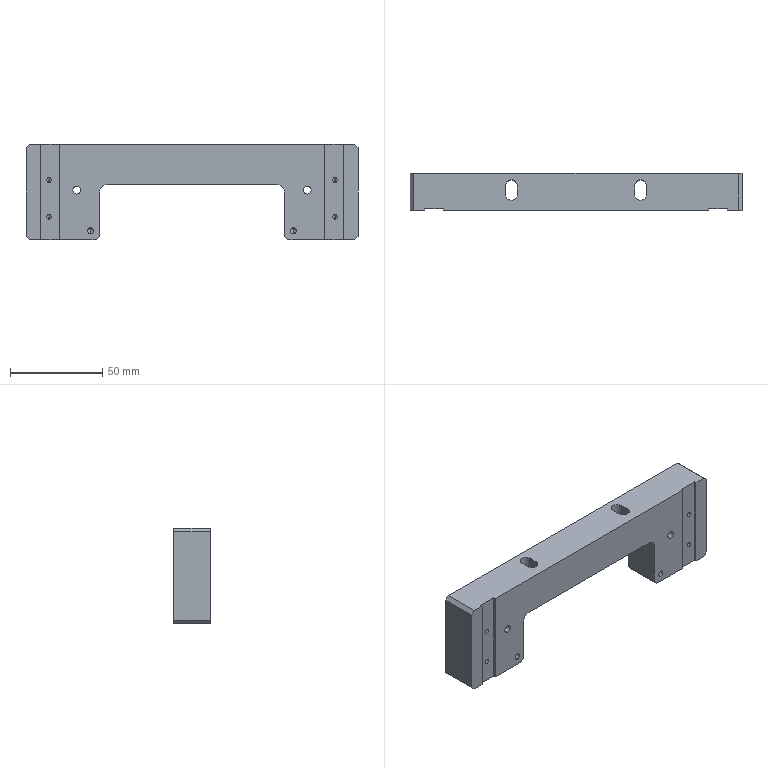Part | STEP file | lift mounting plate 2 | 1 solid | 68 faces | box 180 x 20 x 52 mm | volume 120822 mm3 | plane 30 | cylinder 26 | cone 12 | commonest cylinder face diameters 2.5 x8 3.3 x4 4.2 x4 6.5 x4 11 x4 8 x2